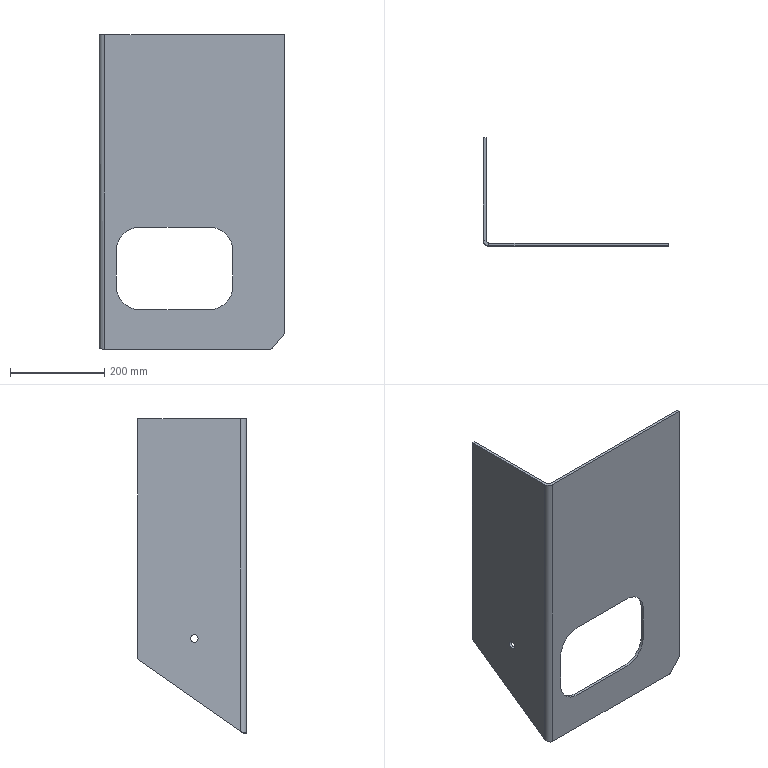Part | SolidWorks | features ICE 3, Chamfer 1, Fillet 1, FlatPattern 1, SMBaseFlange 1, SheetMetal 1 | 1 solid | 28 faces | box 394 x 230 x 667.799 mm | volume 2103650 mm3 | plane 16 | cylinder 11 | spline 1 | commonest cylinder face diameters 100 x4 15 x3 16 x2 12 x1 24 x1
STEP:
#1=CARTESIAN_POINT('',(6.,110.,-122.6));
#2=VERTEX_POINT('',#1);
#3=CARTESIAN_POINT('',(6.,110.,-138.6));
#4=VERTEX_POINT('',#3);
#5=CARTESIAN_POINT('',(6.,110.,-130.6));
#6=DIRECTION('',(1.,0.,0.));
#7=DIRECTION('',(0.,0.,-1.));
#8=AXIS2_PLACEMENT_3D('',#5,#6,#7);
#9=CIRCLE('',#8,8.);
#10=EDGE_CURVE('',#2,#4,#9,.T.);
#11=ORIENTED_EDGE('',*,*,#10,.T.);
#12=CARTESIAN_POINT('',(0.,110.,-138.6));
#13=VERTEX_POINT('',#12);
#14=CARTESIAN_POINT('',(10.,110.,-138.6));
#15=DIRECTION('',(-1.,0.,0.));
#16=VECTOR('',#15,1000.);
#17=LINE('',#14,#16);
#18=EDGE_CURVE('',#4,#13,#17,.T.);
#19=ORIENTED_EDGE('',*,*,#18,.T.);
#20=CARTESIAN_POINT('',(0.,110.,-122.6));
#21=VERTEX_POINT('',#20);
#22=CARTESIAN_POINT('',(0.,110.,-130.6));
#23=DIRECTION('',(-1.,0.,0.));
#24=DIRECTION('',(0.,0.,1.));
#25=AXIS2_PLACEMENT_3D('',#22,#23,#24);
#26=CIRCLE('',#25,8.);
#27=EDGE_CURVE('',#13,#21,#26,.T.);
#28=ORIENTED_EDGE('',*,*,#27,.T.);
#29=CARTESIAN_POINT('',(10.,110.,-122.6));
#30=DIRECTION('',(-1.,0.,0.));
#31=VECTOR('',#30,1000.);
#32=LINE('',#29,#31);
#33=EDGE_CURVE('',#2,#21,#32,.T.);
#34=ORIENTED_EDGE('',*,*,#33,.F.);
#35=EDGE_LOOP('',(#11,#19,#28,#34));
#36=FACE_OUTER_BOUND('',#35,.T.);
#37=CARTESIAN_POINT('',(10.,110.,-130.6));
#38=DIRECTION('',(-1.,0.,0.));
#39=DIRECTION('',(0.,0.,1.));
#40=AXIS2_PLACEMENT_3D('',#37,#38,#39);
#41=CYLINDRICAL_SURFACE('',#40,8.);
#42=ADVANCED_FACE('',(#36),#41,.F.);
#43=CARTESIAN_POINT('',(284.,0.,-197.7));
#44=VERTEX_POINT('',#43);
#45=CARTESIAN_POINT('',(284.,0.,-122.7));
#46=VERTEX_POINT('',#45);
#47=CARTESIAN_POINT('',(284.,0.,-197.7));
#48=DIRECTION('',(0.,0.,1.));
#49=VECTOR('',#48,1000.);
#50=LINE('',#47,#49);
#51=EDGE_CURVE('',#44,#46,#50,.T.);
#52=ORIENTED_EDGE('',*,*,#51,.F.);
#53=CARTESIAN_POINT('',(234.,0.,-247.7));
#54=VERTEX_POINT('',#53);
#55=CARTESIAN_POINT('',(234.,0.,-197.7));
#56=DIRECTION('',(0.,-1.,0.));
#57=DIRECTION('',(0.,0.,-1.));
#58=AXIS2_PLACEMENT_3D('',#55,#56,#57);
#59=CIRCLE('',#58,50.);
#60=EDGE_CURVE('',#54,#44,#59,.T.);
#61=ORIENTED_EDGE('',*,*,#60,.F.);
#62=CARTESIAN_POINT('',(86.,0.,-247.7));
#63=VERTEX_POINT('',#62);
#64=CARTESIAN_POINT('',(86.,0.,-247.7));
#65=DIRECTION('',(1.,0.,0.));
#66=VECTOR('',#65,1000.);
#67=LINE('',#64,#66);
#68=EDGE_CURVE('',#63,#54,#67,.T.);
#69=ORIENTED_EDGE('',*,*,#68,.F.);
#70=CARTESIAN_POINT('',(36.,0.,-197.7));
#71=VERTEX_POINT('',#70);
#72=CARTESIAN_POINT('',(86.,0.,-197.7));
#73=DIRECTION('',(0.,-1.,0.));
#74=DIRECTION('',(0.,0.,1.));
#75=AXIS2_PLACEMENT_3D('',#72,#73,#74);
#76=CIRCLE('',#75,50.);
#77=EDGE_CURVE('',#71,#63,#76,.T.);
#78=ORIENTED_EDGE('',*,*,#77,.F.);
#79=CARTESIAN_POINT('',(36.,0.,-122.7));
#80=VERTEX_POINT('',#79);
#81=CARTESIAN_POINT('',(36.,0.,-197.7));
#82=DIRECTION('',(0.,0.,-1.));
#83=VECTOR('',#82,1000.);
#84=LINE('',#81,#83);
#85=EDGE_CURVE('',#80,#71,#84,.T.);
#86=ORIENTED_EDGE('',*,*,#85,.F.);
#87=CARTESIAN_POINT('',(86.,0.,-72.7));
#88=VERTEX_POINT('',#87);
#89=CARTESIAN_POINT('',(86.,0.,-122.7));
#90=DIRECTION('',(0.,-1.,0.));
#91=DIRECTION('',(0.,0.,1.));
#92=AXIS2_PLACEMENT_3D('',#89,#90,#91);
#93=CIRCLE('',#92,50.);
#94=EDGE_CURVE('',#88,#80,#93,.T.);
#95=ORIENTED_EDGE('',*,*,#94,.F.);
#96=CARTESIAN_POINT('',(234.,0.,-72.7));
#97=VERTEX_POINT('',#96);
#98=CARTESIAN_POINT('',(86.,0.,-72.7));
#99=DIRECTION('',(-1.,0.,0.));
#100=VECTOR('',#99,1000.);
#101=LINE('',#98,#100);
#102=EDGE_CURVE('',#97,#88,#101,.T.);
#103=ORIENTED_EDGE('',*,*,#102,.F.);
#104=CARTESIAN_POINT('',(234.,0.,-122.7));
#105=DIRECTION('',(0.,-1.,0.));
#106=DIRECTION('',(0.,0.,1.));
#107=AXIS2_PLACEMENT_3D('',#104,#105,#106);
#108=CIRCLE('',#107,50.);
#109=EDGE_CURVE('',#46,#97,#108,.T.);
#110=ORIENTED_EDGE('',*,*,#109,.F.);
#111=EDGE_LOOP('',(#52,#61,#69,#78,#86,#95,#103,#110));
#112=FACE_BOUND('',#111,.T.);
#113=CARTESIAN_POINT('',(368.25,0.,-329.067));
#114=VERTEX_POINT('',#113);
#115=CARTESIAN_POINT('',(392.289,0.,-299.876));
#116=VERTEX_POINT('',#115);
#117=CARTESIAN_POINT('',(366.,0.,-331.799));
#118=DIRECTION('',(0.6357,0.,0.7719));
#119=VECTOR('',#118,1000.);
#120=LINE('',#117,#119);
#121=EDGE_CURVE('',#114,#116,#120,.T.);
#122=ORIENTED_EDGE('',*,*,#121,.T.);
#123=CARTESIAN_POINT('',(394.,0.,-295.108));
#124=VERTEX_POINT('',#123);
#125=CARTESIAN_POINT('',(386.5,0.,-295.108));
#126=DIRECTION('',(0.,-1.,0.));
#127=DIRECTION('',(0.,0.,1.));
#128=AXIS2_PLACEMENT_3D('',#125,#126,#127);
#129=CIRCLE('',#128,7.5);
#130=EDGE_CURVE('',#116,#124,#129,.T.);
#131=ORIENTED_EDGE('',*,*,#130,.T.);
#132=CARTESIAN_POINT('',(394.,0.,336.));
#133=VERTEX_POINT('',#132);
#134=CARTESIAN_POINT('',(394.,0.,336.));
#135=DIRECTION('',(0.,0.,-1.));
#136=VECTOR('',#135,1000.);
#137=LINE('',#134,#136);
#138=EDGE_CURVE('',#133,#124,#137,.T.);
#139=ORIENTED_EDGE('',*,*,#138,.F.);
#140=CARTESIAN_POINT('',(12.,0.,336.));
#141=VERTEX_POINT('',#140);
#142=CARTESIAN_POINT('',(0.,0.,336.));
#143=DIRECTION('',(1.,0.,0.));
#144=VECTOR('',#143,1000.);
#145=LINE('',#142,#144);
#146=EDGE_CURVE('',#141,#133,#145,.T.);
#147=ORIENTED_EDGE('',*,*,#146,.F.);
#148=CARTESIAN_POINT('',(12.,0.,-331.799));
#149=VERTEX_POINT('',#148);
#150=CARTESIAN_POINT('',(12.,0.,336.));
#151=DIRECTION('',(0.,0.,-1.));
#152=VECTOR('',#151,1000.);
#153=LINE('',#150,#152);
#154=EDGE_CURVE('',#141,#149,#153,.T.);
#155=ORIENTED_EDGE('',*,*,#154,.T.);
#156=CARTESIAN_POINT('',(362.461,0.,-331.799));
#157=VERTEX_POINT('',#156);
#158=CARTESIAN_POINT('',(0.,0.,-331.799));
#159=DIRECTION('',(1.,0.,0.));
#160=VECTOR('',#159,1000.);
#161=LINE('',#158,#160);
#162=EDGE_CURVE('',#149,#157,#161,.T.);
#163=ORIENTED_EDGE('',*,*,#162,.T.);
#164=CARTESIAN_POINT('',(362.461,0.,-324.299));
#165=DIRECTION('',(0.,-1.,0.));
#166=DIRECTION('',(0.,0.,1.));
#167=AXIS2_PLACEMENT_3D('',#164,#165,#166);
#168=CIRCLE('',#167,7.5);
#169=EDGE_CURVE('',#157,#114,#168,.T.);
#170=ORIENTED_EDGE('',*,*,#169,.T.);
#171=EDGE_LOOP('',(#122,#131,#139,#147,#155,#163,#170));
#172=FACE_OUTER_BOUND('',#171,.T.);
#173=CARTESIAN_POINT('',(0.,0.,336.));
#174=DIRECTION('',(0.,1.,0.));
#175=DIRECTION('',(0.,0.,1.));
#176=AXIS2_PLACEMENT_3D('',#173,#174,#175);
#177=PLANE('',#176);
#178=ADVANCED_FACE('',(#112,#172),#177,.F.);
#179=ORIENTED_EDGE('',*,*,#138,.T.);
#180=CARTESIAN_POINT('',(394.,6.,-295.108));
#181=VERTEX_POINT('',#180);
#182=CARTESIAN_POINT('',(394.,6.,-295.108));
#183=DIRECTION('',(0.,1.,0.));
#184=VECTOR('',#183,1000.);
#185=LINE('',#182,#184);
#186=EDGE_CURVE('',#124,#181,#185,.T.);
#187=ORIENTED_EDGE('',*,*,#186,.T.);
#188=CARTESIAN_POINT('',(394.,6.,336.));
#189=VERTEX_POINT('',#188);
#190=CARTESIAN_POINT('',(394.,6.,336.));
#191=DIRECTION('',(0.,0.,-1.));
#192=VECTOR('',#191,1000.);
#193=LINE('',#190,#192);
#194=EDGE_CURVE('',#189,#181,#193,.T.);
#195=ORIENTED_EDGE('',*,*,#194,.F.);
#196=CARTESIAN_POINT('',(394.,6.,336.));
#197=DIRECTION('',(0.,-1.,0.));
#198=VECTOR('',#197,1000.);
#199=LINE('',#196,#198);
#200=EDGE_CURVE('',#189,#133,#199,.T.);
#201=ORIENTED_EDGE('',*,*,#200,.T.);
#202=EDGE_LOOP('',(#179,#187,#195,#201));
#203=FACE_OUTER_BOUND('',#202,.T.);
#204=CARTESIAN_POINT('',(394.,6.,336.));
#205=DIRECTION('',(1.,0.,0.));
#206=DIRECTION('',(0.,0.,-1.));
#207=AXIS2_PLACEMENT_3D('',#204,#205,#206);
#208=PLANE('',#207);
#209=ADVANCED_FACE('',(#203),#208,.T.);
#210=CARTESIAN_POINT('',(284.,6.,-197.7));
#211=VERTEX_POINT('',#210);
#212=CARTESIAN_POINT('',(234.,6.,-247.7));
#213=VERTEX_POINT('',#212);
#214=CARTESIAN_POINT('',(234.,6.,-197.7));
#215=DIRECTION('',(0.,1.,0.));
#216=DIRECTION('',(0.,0.,1.));
#217=AXIS2_PLACEMENT_3D('',#214,#215,#216);
#218=CIRCLE('',#217,50.);
#219=EDGE_CURVE('',#211,#213,#218,.T.);
#220=ORIENTED_EDGE('',*,*,#219,.F.);
#221=CARTESIAN_POINT('',(284.,6.,-122.7));
#222=VERTEX_POINT('',#221);
#223=CARTESIAN_POINT('',(284.,6.,336.));
#224=DIRECTION('',(0.,0.,-1.));
#225=VECTOR('',#224,1000.);
#226=LINE('',#223,#225);
#227=EDGE_CURVE('',#222,#211,#226,.T.);
#228=ORIENTED_EDGE('',*,*,#227,.F.);
#229=CARTESIAN_POINT('',(234.,6.,-72.7));
#230=VERTEX_POINT('',#229);
#231=CARTESIAN_POINT('',(234.,6.,-122.7));
#232=DIRECTION('',(0.,1.,0.));
#233=DIRECTION('',(0.,0.,1.));
#234=AXIS2_PLACEMENT_3D('',#231,#232,#233);
#235=CIRCLE('',#234,50.);
#236=EDGE_CURVE('',#230,#222,#235,.T.);
#237=ORIENTED_EDGE('',*,*,#236,.F.);
#238=CARTESIAN_POINT('',(86.,6.,-72.7));
#239=VERTEX_POINT('',#238);
#240=CARTESIAN_POINT('',(0.,6.,-72.7));
#241=DIRECTION('',(1.,0.,0.));
#242=VECTOR('',#241,1000.);
#243=LINE('',#240,#242);
#244=EDGE_CURVE('',#239,#230,#243,.T.);
#245=ORIENTED_EDGE('',*,*,#244,.F.);
#246=CARTESIAN_POINT('',(36.,6.,-122.7));
#247=VERTEX_POINT('',#246);
#248=CARTESIAN_POINT('',(86.,6.,-122.7));
#249=DIRECTION('',(0.,1.,0.));
#250=DIRECTION('',(0.,0.,1.));
#251=AXIS2_PLACEMENT_3D('',#248,#249,#250);
#252=CIRCLE('',#251,50.);
#253=EDGE_CURVE('',#247,#239,#252,.T.);
#254=ORIENTED_EDGE('',*,*,#253,.F.);
#255=CARTESIAN_POINT('',(36.,6.,-197.7));
#256=VERTEX_POINT('',#255);
#257=CARTESIAN_POINT('',(36.,6.,336.));
#258=DIRECTION('',(0.,0.,1.));
#259=VECTOR('',#258,1000.);
#260=LINE('',#257,#259);
#261=EDGE_CURVE('',#256,#247,#260,.T.);
#262=ORIENTED_EDGE('',*,*,#261,.F.);
#263=CARTESIAN_POINT('',(86.,6.,-247.7));
#264=VERTEX_POINT('',#263);
#265=CARTESIAN_POINT('',(86.,6.,-197.7));
#266=DIRECTION('',(0.,1.,0.));
#267=DIRECTION('',(0.,0.,1.));
#268=AXIS2_PLACEMENT_3D('',#265,#266,#267);
#269=CIRCLE('',#268,50.);
#270=EDGE_CURVE('',#264,#256,#269,.T.);
#271=ORIENTED_EDGE('',*,*,#270,.F.);
#272=CARTESIAN_POINT('',(0.,6.,-247.7));
#273=DIRECTION('',(-1.,0.,0.));
#274=VECTOR('',#273,1000.);
#275=LINE('',#272,#274);
#276=EDGE_CURVE('',#213,#264,#275,.T.);
#277=ORIENTED_EDGE('',*,*,#276,.F.);
#278=EDGE_LOOP('',(#220,#228,#237,#245,#254,#262,#271,#277));
#279=FACE_BOUND('',#278,.T.);
#280=ORIENTED_EDGE('',*,*,#194,.T.);
#281=CARTESIAN_POINT('',(392.289,6.,-299.876));
#282=VERTEX_POINT('',#281);
#283=CARTESIAN_POINT('',(386.5,6.,-295.108));
#284=DIRECTION('',(0.,1.,0.));
#285=DIRECTION('',(0.,0.,1.));
#286=AXIS2_PLACEMENT_3D('',#283,#284,#285);
#287=CIRCLE('',#286,7.5);
#288=EDGE_CURVE('',#181,#282,#287,.T.);
#289=ORIENTED_EDGE('',*,*,#288,.T.);
#290=CARTESIAN_POINT('',(368.25,6.,-329.067));
#291=VERTEX_POINT('',#290);
#292=CARTESIAN_POINT('',(545.794,6.,-113.477));
#293=DIRECTION('',(-0.6357,0.,-0.7719));
#294=VECTOR('',#293,1000.);
#295=LINE('',#292,#294);
#296=EDGE_CURVE('',#282,#291,#295,.T.);
#297=ORIENTED_EDGE('',*,*,#296,.T.);
#298=CARTESIAN_POINT('',(362.461,6.,-331.799));
#299=VERTEX_POINT('',#298);
#300=CARTESIAN_POINT('',(362.461,6.,-324.299));
#301=DIRECTION('',(0.,1.,0.));
#302=DIRECTION('',(0.,0.,1.));
#303=AXIS2_PLACEMENT_3D('',#300,#301,#302);
#304=CIRCLE('',#303,7.5);
#305=EDGE_CURVE('',#291,#299,#304,.T.);
#306=ORIENTED_EDGE('',*,*,#305,.T.);
#307=CARTESIAN_POINT('',(12.,6.,-331.799));
#308=VERTEX_POINT('',#307);
#309=CARTESIAN_POINT('',(0.,6.,-331.799));
#310=DIRECTION('',(1.,0.,0.));
#311=VECTOR('',#310,1000.);
#312=LINE('',#309,#311);
#313=EDGE_CURVE('',#308,#299,#312,.T.);
#314=ORIENTED_EDGE('',*,*,#313,.F.);
#315=CARTESIAN_POINT('',(12.,6.,336.));
#316=VERTEX_POINT('',#315);
#317=CARTESIAN_POINT('',(12.,6.,336.));
#318=DIRECTION('',(0.,0.,-1.));
#319=VECTOR('',#318,1000.);
#320=LINE('',#317,#319);
#321=EDGE_CURVE('',#316,#308,#320,.T.);
#322=ORIENTED_EDGE('',*,*,#321,.F.);
#323=CARTESIAN_POINT('',(0.,6.,336.));
#324=DIRECTION('',(1.,0.,0.));
#325=VECTOR('',#324,1000.);
#326=LINE('',#323,#325);
#327=EDGE_CURVE('',#316,#189,#326,.T.);
#328=ORIENTED_EDGE('',*,*,#327,.T.);
#329=EDGE_LOOP('',(#280,#289,#297,#306,#314,#322,#328));
#330=FACE_OUTER_BOUND('',#329,.T.);
#331=CARTESIAN_POINT('',(0.,6.,336.));
#332=DIRECTION('',(0.,1.,0.));
#333=DIRECTION('',(0.,0.,1.));
#334=AXIS2_PLACEMENT_3D('',#331,#332,#333);
#335=PLANE('',#334);
#336=ADVANCED_FACE('',(#279,#330),#335,.T.);
#337=ORIENTED_EDGE('',*,*,#321,.T.);
#338=CARTESIAN_POINT('',(6.,12.,-327.598));
#339=VERTEX_POINT('',#338);
#340=CARTESIAN_POINT('',(6.,12.,-327.598));
#341=CARTESIAN_POINT('',(6.,8.485,-330.059));
#342=CARTESIAN_POINT('',(8.485,6.,-331.799));
#343=CARTESIAN_POINT('',(12.,6.,-331.799));
#344=(BOUNDED_CURVE()B_SPLINE_CURVE(3,(#340,#341,#342,#343),.UNSPECIFIED.,.F.,.T.)B_SPLINE_CURVE_WITH_KNOTS((4,4),(4.712,6.283),.UNSPECIFIED.)CURVE()GEOMETRIC_REPRESENTATION_ITEM()RATIONAL_B_SPLINE_CURVE((1.,0.8047,0.8047,1.))REPRESENTATION_ITEM(''));
#345=EDGE_CURVE('',#339,#308,#344,.T.);
#346=ORIENTED_EDGE('',*,*,#345,.F.);
#347=CARTESIAN_POINT('',(6.,12.,336.));
#348=VERTEX_POINT('',#347);
#349=CARTESIAN_POINT('',(6.,12.,336.));
#350=DIRECTION('',(0.,0.,-1.));
#351=VECTOR('',#350,1000.);
#352=LINE('',#349,#351);
#353=EDGE_CURVE('',#348,#339,#352,.T.);
#354=ORIENTED_EDGE('',*,*,#353,.F.);
#355=CARTESIAN_POINT('',(12.,12.,336.));
#356=DIRECTION('',(0.,0.,1.));
#357=DIRECTION('',(1.,0.,0.));
#358=AXIS2_PLACEMENT_3D('',#355,#356,#357);
#359=CIRCLE('',#358,6.);
#360=EDGE_CURVE('',#348,#316,#359,.T.);
#361=ORIENTED_EDGE('',*,*,#360,.T.);
#362=EDGE_LOOP('',(#337,#346,#354,#361));
#363=FACE_OUTER_BOUND('',#362,.T.);
#364=CARTESIAN_POINT('',(12.,12.,336.));
#365=DIRECTION('',(0.,0.,-1.));
#366=DIRECTION('',(-1.,0.,0.));
#367=AXIS2_PLACEMENT_3D('',#364,#365,#366);
#368=CYLINDRICAL_SURFACE('',#367,6.);
#369=ADVANCED_FACE('',(#363),#368,.F.);
#370=ORIENTED_EDGE('',*,*,#10,.F.);
#371=CARTESIAN_POINT('',(6.,110.,-130.6));
#372=DIRECTION('',(1.,0.,0.));
#373=DIRECTION('',(0.,0.,-1.));
#374=AXIS2_PLACEMENT_3D('',#371,#372,#373);
#375=CIRCLE('',#374,8.);
#376=EDGE_CURVE('',#4,#2,#375,.T.);
#377=ORIENTED_EDGE('',*,*,#376,.F.);
#378=EDGE_LOOP('',(#370,#377));
#379=FACE_BOUND('',#378,.T.);
#380=CARTESIAN_POINT('',(6.,226.802,-177.192));
#381=VERTEX_POINT('',#380);
#382=CARTESIAN_POINT('',(6.,315.737,-114.919));
#383=DIRECTION('',(0.,-0.8192,-0.5736));
#384=VECTOR('',#383,1000.);
#385=LINE('',#382,#384);
#386=EDGE_CURVE('',#381,#339,#385,.T.);
#387=ORIENTED_EDGE('',*,*,#386,.F.);
#388=CARTESIAN_POINT('',(6.,230.,-171.048));
#389=VERTEX_POINT('',#388);
#390=CARTESIAN_POINT('',(6.,222.5,-171.048));
#391=DIRECTION('',(1.,0.,0.));
#392=DIRECTION('',(0.,0.,-1.));
#393=AXIS2_PLACEMENT_3D('',#390,#391,#392);
#394=CIRCLE('',#393,7.5);
#395=EDGE_CURVE('',#381,#389,#394,.T.);
#396=ORIENTED_EDGE('',*,*,#395,.T.);
#397=CARTESIAN_POINT('',(6.,230.,336.));
#398=VERTEX_POINT('',#397);
#399=CARTESIAN_POINT('',(6.,230.,336.));
#400=DIRECTION('',(0.,0.,-1.));
#401=VECTOR('',#400,1000.);
#402=LINE('',#399,#401);
#403=EDGE_CURVE('',#398,#389,#402,.T.);
#404=ORIENTED_EDGE('',*,*,#403,.F.);
#405=CARTESIAN_POINT('',(6.,0.,336.));
#406=DIRECTION('',(0.,-1.,0.));
#407=VECTOR('',#406,1000.);
#408=LINE('',#405,#407);
#409=EDGE_CURVE('',#398,#348,#408,.T.);
#410=ORIENTED_EDGE('',*,*,#409,.T.);
#411=ORIENTED_EDGE('',*,*,#353,.T.);
#412=EDGE_LOOP('',(#387,#396,#404,#410,#411));
#413=FACE_OUTER_BOUND('',#412,.T.);
#414=CARTESIAN_POINT('',(6.,0.,336.));
#415=DIRECTION('',(1.,0.,0.));
#416=DIRECTION('',(0.,0.,-1.));
#417=AXIS2_PLACEMENT_3D('',#414,#415,#416);
#418=PLANE('',#417);
#419=ADVANCED_FACE('',(#379,#413),#418,.T.);
#420=ORIENTED_EDGE('',*,*,#403,.T.);
#421=CARTESIAN_POINT('',(0.,230.,-171.048));
#422=VERTEX_POINT('',#421);
#423=CARTESIAN_POINT('',(0.,230.,-171.048));
#424=DIRECTION('',(-1.,0.,0.));
#425=VECTOR('',#424,1000.);
#426=LINE('',#423,#425);
#427=EDGE_CURVE('',#389,#422,#426,.T.);
#428=ORIENTED_EDGE('',*,*,#427,.T.);
#429=CARTESIAN_POINT('',(0.,230.,336.));
#430=VERTEX_POINT('',#429);
#431=CARTESIAN_POINT('',(0.,230.,336.));
#432=DIRECTION('',(0.,0.,-1.));
#433=VECTOR('',#432,1000.);
#434=LINE('',#431,#433);
#435=EDGE_CURVE('',#430,#422,#434,.T.);
#436=ORIENTED_EDGE('',*,*,#435,.F.);
#437=CARTESIAN_POINT('',(0.,230.,336.));
#438=DIRECTION('',(1.,0.,0.));
#439=VECTOR('',#438,1000.);
#440=LINE('',#437,#439);
#441=EDGE_CURVE('',#430,#398,#440,.T.);
#442=ORIENTED_EDGE('',*,*,#441,.T.);
#443=EDGE_LOOP('',(#420,#428,#436,#442));
#444=FACE_OUTER_BOUND('',#443,.T.);
#445=CARTESIAN_POINT('',(0.,230.,336.));
#446=DIRECTION('',(0.,1.,0.));
#447=DIRECTION('',(0.,0.,1.));
#448=AXIS2_PLACEMENT_3D('',#445,#446,#447);
#449=PLANE('',#448);
#450=ADVANCED_FACE('',(#444),#449,.T.);
#451=CARTESIAN_POINT('',(0.,110.,-130.6));
#452=DIRECTION('',(-1.,0.,0.));
#453=DIRECTION('',(0.,0.,1.));
#454=AXIS2_PLACEMENT_3D('',#451,#452,#453);
#455=CIRCLE('',#454,8.);
#456=EDGE_CURVE('',#21,#13,#455,.T.);
#457=ORIENTED_EDGE('',*,*,#456,.F.);
#458=ORIENTED_EDGE('',*,*,#27,.F.);
#459=EDGE_LOOP('',(#457,#458));
#460=FACE_BOUND('',#459,.T.);
#461=ORIENTED_EDGE('',*,*,#435,.T.);
#462=CARTESIAN_POINT('',(0.,226.802,-177.192));
#463=VERTEX_POINT('',#462);
#464=CARTESIAN_POINT('',(0.,222.5,-171.048));
#465=DIRECTION('',(-1.,0.,0.));
#466=DIRECTION('',(0.,0.,-1.));
#467=AXIS2_PLACEMENT_3D('',#464,#465,#466);
#468=CIRCLE('',#467,7.5);
#469=EDGE_CURVE('',#422,#463,#468,.T.);
#470=ORIENTED_EDGE('',*,*,#469,.T.);
#471=CARTESIAN_POINT('',(0.,12.,-327.598));
#472=VERTEX_POINT('',#471);
#473=CARTESIAN_POINT('',(0.,315.737,-114.919));
#474=DIRECTION('',(0.,-0.8192,-0.5736));
#475=VECTOR('',#474,1000.);
#476=LINE('',#473,#475);
#477=EDGE_CURVE('',#463,#472,#476,.T.);
#478=ORIENTED_EDGE('',*,*,#477,.T.);
#479=CARTESIAN_POINT('',(0.,12.,336.));
#480=VERTEX_POINT('',#479);
#481=CARTESIAN_POINT('',(0.,12.,336.));
#482=DIRECTION('',(0.,0.,-1.));
#483=VECTOR('',#482,1000.);
#484=LINE('',#481,#483);
#485=EDGE_CURVE('',#480,#472,#484,.T.);
#486=ORIENTED_EDGE('',*,*,#485,.F.);
#487=CARTESIAN_POINT('',(0.,0.,336.));
#488=DIRECTION('',(0.,-1.,0.));
#489=VECTOR('',#488,1000.);
#490=LINE('',#487,#489);
#491=EDGE_CURVE('',#430,#480,#490,.T.);
#492=ORIENTED_EDGE('',*,*,#491,.F.);
#493=EDGE_LOOP('',(#461,#470,#478,#486,#492));
#494=FACE_OUTER_BOUND('',#493,.T.);
#495=CARTESIAN_POINT('',(0.,0.,336.));
#496=DIRECTION('',(1.,0.,0.));
#497=DIRECTION('',(0.,0.,-1.));
#498=AXIS2_PLACEMENT_3D('',#495,#496,#497);
#499=PLANE('',#498);
#500=ADVANCED_FACE('',(#460,#494),#499,.F.);
#501=CARTESIAN_POINT('',(0.,12.,-327.598));
#502=CARTESIAN_POINT('',(0.,4.971,-330.059));
#503=CARTESIAN_POINT('',(4.971,0.,-331.799));
#504=CARTESIAN_POINT('',(12.,0.,-331.799));
#505=(BOUNDED_CURVE()B_SPLINE_CURVE(3,(#501,#502,#503,#504),.UNSPECIFIED.,.F.,.F.)B_SPLINE_CURVE_WITH_KNOTS((4,4),(4.712,6.283),.UNSPECIFIED.)CURVE()GEOMETRIC_REPRESENTATION_ITEM()RATIONAL_B_SPLINE_CURVE((1.,0.8047,0.8047,1.))REPRESENTATION_ITEM(''));
#506=EDGE_CURVE('',#472,#149,#505,.T.);
#507=ORIENTED_EDGE('',*,*,#506,.T.);
#508=ORIENTED_EDGE('',*,*,#154,.F.);
#509=CARTESIAN_POINT('',(12.,12.,336.));
#510=DIRECTION('',(0.,0.,1.));
#511=DIRECTION('',(-1.,0.,0.));
#512=AXIS2_PLACEMENT_3D('',#509,#510,#511);
#513=CIRCLE('',#512,12.);
#514=EDGE_CURVE('',#480,#141,#513,.T.);
#515=ORIENTED_EDGE('',*,*,#514,.F.);
#516=ORIENTED_EDGE('',*,*,#485,.T.);
#517=EDGE_LOOP('',(#507,#508,#515,#516));
#518=FACE_OUTER_BOUND('',#517,.T.);
#519=CARTESIAN_POINT('',(12.,12.,336.));
#520=DIRECTION('',(0.,0.,-1.));
#521=DIRECTION('',(-1.,0.,0.));
#522=AXIS2_PLACEMENT_3D('',#519,#520,#521);
#523=CYLINDRICAL_SURFACE('',#522,12.);
#524=ADVANCED_FACE('',(#518),#523,.T.);
#525=CARTESIAN_POINT('',(0.,12.,336.));
#526=DIRECTION('',(1.,0.,0.));
#527=VECTOR('',#526,1000.);
#528=LINE('',#525,#527);
#529=EDGE_CURVE('',#480,#348,#528,.T.);
#530=ORIENTED_EDGE('',*,*,#529,.F.);
#531=ORIENTED_EDGE('',*,*,#514,.T.);
#532=CARTESIAN_POINT('',(12.,6.,336.));
#533=DIRECTION('',(0.,-1.,0.));
#534=VECTOR('',#533,1000.);
#535=LINE('',#532,#534);
#536=EDGE_CURVE('',#316,#141,#535,.T.);
#537=ORIENTED_EDGE('',*,*,#536,.F.);
#538=ORIENTED_EDGE('',*,*,#360,.F.);
#539=EDGE_LOOP('',(#530,#531,#537,#538));
#540=FACE_OUTER_BOUND('',#539,.T.);
#541=CARTESIAN_POINT('',(0.,12.,336.));
#542=DIRECTION('',(0.,0.,1.));
#543=DIRECTION('',(1.,0.,0.));
#544=AXIS2_PLACEMENT_3D('',#541,#542,#543);
#545=PLANE('',#544);
#546=ADVANCED_FACE('',(#540),#545,.T.);
#547=ORIENTED_EDGE('',*,*,#491,.T.);
#548=ORIENTED_EDGE('',*,*,#529,.T.);
#549=ORIENTED_EDGE('',*,*,#409,.F.);
#550=ORIENTED_EDGE('',*,*,#441,.F.);
#551=EDGE_LOOP('',(#547,#548,#549,#550));
#552=FACE_OUTER_BOUND('',#551,.T.);
#553=CARTESIAN_POINT('',(12.,6.,336.));
#554=DIRECTION('',(0.,0.,1.));
#555=DIRECTION('',(1.,0.,0.));
#556=AXIS2_PLACEMENT_3D('',#553,#554,#555);
#557=PLANE('',#556);
#558=ADVANCED_FACE('',(#552),#557,.T.);
#559=ORIENTED_EDGE('',*,*,#146,.T.);
#560=ORIENTED_EDGE('',*,*,#200,.F.);
#561=ORIENTED_EDGE('',*,*,#327,.F.);
#562=ORIENTED_EDGE('',*,*,#536,.T.);
#563=EDGE_LOOP('',(#559,#560,#561,#562));
#564=FACE_OUTER_BOUND('',#563,.T.);
#565=CARTESIAN_POINT('',(12.,12.,336.));
#566=DIRECTION('',(0.,0.,1.));
#567=DIRECTION('',(1.,0.,0.));
#568=AXIS2_PLACEMENT_3D('',#565,#566,#567);
#569=PLANE('',#568);
#570=ADVANCED_FACE('',(#564),#569,.T.);
#571=ORIENTED_EDGE('',*,*,#313,.T.);
#572=CARTESIAN_POINT('',(362.461,6.,-331.799));
#573=DIRECTION('',(0.,-1.,0.));
#574=VECTOR('',#573,1000.);
#575=LINE('',#572,#574);
#576=EDGE_CURVE('',#299,#157,#575,.T.);
#577=ORIENTED_EDGE('',*,*,#576,.T.);
#578=ORIENTED_EDGE('',*,*,#162,.F.);
#579=CARTESIAN_POINT('',(12.,6.,-331.799));
#580=DIRECTION('',(0.,-1.,0.));
#581=VECTOR('',#580,1000.);
#582=LINE('',#579,#581);
#583=EDGE_CURVE('',#308,#149,#582,.T.);
#584=ORIENTED_EDGE('',*,*,#583,.F.);
#585=EDGE_LOOP('',(#571,#577,#578,#584));
#586=FACE_OUTER_BOUND('',#585,.T.);
#587=CARTESIAN_POINT('',(0.,6.,-331.799));
#588=DIRECTION('',(0.,0.,1.));
#589=DIRECTION('',(1.,0.,0.));
#590=AXIS2_PLACEMENT_3D('',#587,#588,#589);
#591=PLANE('',#590);
#592=ADVANCED_FACE('',(#586),#591,.F.);
#593=ORIENTED_EDGE('',*,*,#477,.F.);
#594=CARTESIAN_POINT('',(6.,226.802,-177.192));
#595=DIRECTION('',(1.,0.,0.));
#596=VECTOR('',#595,1000.);
#597=LINE('',#594,#596);
#598=EDGE_CURVE('',#463,#381,#597,.T.);
#599=ORIENTED_EDGE('',*,*,#598,.T.);
#600=ORIENTED_EDGE('',*,*,#386,.T.);
#601=CARTESIAN_POINT('',(6.,12.,-327.598));
#602=DIRECTION('',(-1.,0.,0.));
#603=VECTOR('',#602,1000.);
#604=LINE('',#601,#603);
#605=EDGE_CURVE('',#339,#472,#604,.T.);
#606=ORIENTED_EDGE('',*,*,#605,.T.);
#607=EDGE_LOOP('',(#593,#599,#600,#606));
#608=FACE_OUTER_BOUND('',#607,.T.);
#609=CARTESIAN_POINT('',(6.,315.737,-114.919));
#610=DIRECTION('',(0.,-0.5736,0.8192));
#611=DIRECTION('',(0.,-0.8192,-0.5736));
#612=AXIS2_PLACEMENT_3D('',#609,#610,#611);
#613=PLANE('',#612);
#614=ADVANCED_FACE('',(#608),#613,.F.);
#615=ORIENTED_EDGE('',*,*,#345,.T.);
#616=ORIENTED_EDGE('',*,*,#583,.T.);
#617=ORIENTED_EDGE('',*,*,#506,.F.);
#618=ORIENTED_EDGE('',*,*,#605,.F.);
#619=EDGE_LOOP('',(#615,#616,#617,#618));
#620=FACE_OUTER_BOUND('',#619,.T.);
#621=CARTESIAN_POINT('',(12.,6.,-331.799));
#622=CARTESIAN_POINT('',(12.,4.,-331.799));
#623=CARTESIAN_POINT('',(12.,2.,-331.799));
#624=CARTESIAN_POINT('',(12.,0.,-331.799));
#625=CARTESIAN_POINT('',(24.,6.,-331.799));
#626=CARTESIAN_POINT('',(28.,4.,-331.799));
#627=CARTESIAN_POINT('',(32.,2.,-331.799));
#628=CARTESIAN_POINT('',(36.,0.,-331.799));
#629=CARTESIAN_POINT('',(24.,18.,-323.396));
#630=CARTESIAN_POINT('',(28.,20.,-323.396));
#631=CARTESIAN_POINT('',(32.,22.,-323.396));
#632=CARTESIAN_POINT('',(36.,24.,-323.396));
#633=CARTESIAN_POINT('',(12.,18.,-323.396));
#634=CARTESIAN_POINT('',(12.,20.,-323.396));
#635=CARTESIAN_POINT('',(12.,22.,-323.396));
#636=CARTESIAN_POINT('',(12.,24.,-323.396));
#637=CARTESIAN_POINT('',(0.,18.,-323.396));
#638=CARTESIAN_POINT('',(-4.,20.,-323.396));
#639=CARTESIAN_POINT('',(-8.,22.,-323.396));
#640=CARTESIAN_POINT('',(-12.,24.,-323.396));
#641=CARTESIAN_POINT('',(0.,6.,-331.799));
#642=CARTESIAN_POINT('',(-4.,4.,-331.799));
#643=CARTESIAN_POINT('',(-8.,2.,-331.799));
#644=CARTESIAN_POINT('',(-12.,0.,-331.799));
#645=CARTESIAN_POINT('',(12.,6.,-331.799));
#646=CARTESIAN_POINT('',(12.,4.,-331.799));
#647=CARTESIAN_POINT('',(12.,2.,-331.799));
#648=CARTESIAN_POINT('',(12.,0.,-331.799));
#649=(BOUNDED_SURFACE()B_SPLINE_SURFACE(3,3,((#621,#622,#623,#624),(#625,#626,#627,#628),(#629,#630,#631,#632),(#633,#634,#635,#636),(#637,#638,#639,#640),(#641,#642,#643,#644),(#645,#646,#647,#648)),.UNSPECIFIED.,.T.,.F.,.T.)B_SPLINE_SURFACE_WITH_KNOTS((4,3,4),(4,4),(0.,0.5,1.),(0.,1.),.UNSPECIFIED.)GEOMETRIC_REPRESENTATION_ITEM()RATIONAL_B_SPLINE_SURFACE(((1.,1.,1.,1.),(0.3333,0.3333,0.3333,0.3333),(0.3333,0.3333,0.3333,0.3333),(1.,1.,1.,1.),(0.3333,0.3333,0.3333,0.3333),(0.3333,0.3333,0.3333,0.3333),(1.,1.,1.,1.)))REPRESENTATION_ITEM('')SURFACE());
#650=ADVANCED_FACE('',(#620),#649,.T.);
#651=ORIENTED_EDGE('',*,*,#296,.F.);
#652=CARTESIAN_POINT('',(392.289,6.,-299.876));
#653=DIRECTION('',(0.,-1.,0.));
#654=VECTOR('',#653,1000.);
#655=LINE('',#652,#654);
#656=EDGE_CURVE('',#282,#116,#655,.T.);
#657=ORIENTED_EDGE('',*,*,#656,.T.);
#658=ORIENTED_EDGE('',*,*,#121,.F.);
#659=CARTESIAN_POINT('',(368.25,6.,-329.067));
#660=DIRECTION('',(0.,1.,0.));
#661=VECTOR('',#660,1000.);
#662=LINE('',#659,#661);
#663=EDGE_CURVE('',#114,#291,#662,.T.);
#664=ORIENTED_EDGE('',*,*,#663,.T.);
#665=EDGE_LOOP('',(#651,#657,#658,#664));
#666=FACE_OUTER_BOUND('',#665,.T.);
#667=CARTESIAN_POINT('',(366.,6.,-331.799));
#668=DIRECTION('',(0.7719,0.,-0.6357));
#669=DIRECTION('',(0.,1.,0.));
#670=AXIS2_PLACEMENT_3D('',#667,#668,#669);
#671=PLANE('',#670);
#672=ADVANCED_FACE('',(#666),#671,.T.);
#673=ORIENTED_EDGE('',*,*,#395,.F.);
#674=ORIENTED_EDGE('',*,*,#598,.F.);
#675=ORIENTED_EDGE('',*,*,#469,.F.);
#676=ORIENTED_EDGE('',*,*,#427,.F.);
#677=EDGE_LOOP('',(#673,#674,#675,#676));
#678=FACE_OUTER_BOUND('',#677,.T.);
#679=CARTESIAN_POINT('',(0.,222.5,-171.048));
#680=DIRECTION('',(1.,0.,0.));
#681=DIRECTION('',(0.,0.,-1.));
#682=AXIS2_PLACEMENT_3D('',#679,#680,#681);
#683=CYLINDRICAL_SURFACE('',#682,7.5);
#684=ADVANCED_FACE('',(#678),#683,.T.);
#685=ORIENTED_EDGE('',*,*,#130,.F.);
#686=ORIENTED_EDGE('',*,*,#656,.F.);
#687=ORIENTED_EDGE('',*,*,#288,.F.);
#688=ORIENTED_EDGE('',*,*,#186,.F.);
#689=EDGE_LOOP('',(#685,#686,#687,#688));
#690=FACE_OUTER_BOUND('',#689,.T.);
#691=CARTESIAN_POINT('',(386.5,6.,-295.108));
#692=DIRECTION('',(0.,1.,0.));
#693=DIRECTION('',(0.,0.,1.));
#694=AXIS2_PLACEMENT_3D('',#691,#692,#693);
#695=CYLINDRICAL_SURFACE('',#694,7.5);
#696=ADVANCED_FACE('',(#690),#695,.T.);
#697=ORIENTED_EDGE('',*,*,#305,.F.);
#698=ORIENTED_EDGE('',*,*,#663,.F.);
#699=ORIENTED_EDGE('',*,*,#169,.F.);
#700=ORIENTED_EDGE('',*,*,#576,.F.);
#701=EDGE_LOOP('',(#697,#698,#699,#700));
#702=FACE_OUTER_BOUND('',#701,.T.);
#703=CARTESIAN_POINT('',(362.461,6.,-324.299));
#704=DIRECTION('',(0.,1.,0.));
#705=DIRECTION('',(0.,0.,1.));
#706=AXIS2_PLACEMENT_3D('',#703,#704,#705);
#707=CYLINDRICAL_SURFACE('',#706,7.5);
#708=ADVANCED_FACE('',(#702),#707,.T.);
#709=ORIENTED_EDGE('',*,*,#18,.F.);
#710=ORIENTED_EDGE('',*,*,#376,.T.);
#711=ORIENTED_EDGE('',*,*,#33,.T.);
#712=ORIENTED_EDGE('',*,*,#456,.T.);
#713=EDGE_LOOP('',(#709,#710,#711,#712));
#714=FACE_OUTER_BOUND('',#713,.T.);
#715=CARTESIAN_POINT('',(10.,110.,-130.6));
#716=DIRECTION('',(-1.,0.,0.));
#717=DIRECTION('',(0.,0.,1.));
#718=AXIS2_PLACEMENT_3D('',#715,#716,#717);
#719=CYLINDRICAL_SURFACE('',#718,8.);
#720=ADVANCED_FACE('',(#714),#719,.F.);
#721=ORIENTED_EDGE('',*,*,#219,.T.);
#722=CARTESIAN_POINT('',(234.,10.,-247.7));
#723=DIRECTION('',(0.,-1.,0.));
#724=VECTOR('',#723,1000.);
#725=LINE('',#722,#724);
#726=EDGE_CURVE('',#213,#54,#725,.T.);
#727=ORIENTED_EDGE('',*,*,#726,.T.);
#728=ORIENTED_EDGE('',*,*,#60,.T.);
#729=CARTESIAN_POINT('',(284.,10.,-197.7));
#730=DIRECTION('',(0.,-1.,0.));
#731=VECTOR('',#730,1000.);
#732=LINE('',#729,#731);
#733=EDGE_CURVE('',#211,#44,#732,.T.);
#734=ORIENTED_EDGE('',*,*,#733,.F.);
#735=EDGE_LOOP('',(#721,#727,#728,#734));
#736=FACE_OUTER_BOUND('',#735,.T.);
#737=CARTESIAN_POINT('',(234.,10.,-197.7));
#738=DIRECTION('',(0.,-1.,0.));
#739=DIRECTION('',(0.,0.,-1.));
#740=AXIS2_PLACEMENT_3D('',#737,#738,#739);
#741=CYLINDRICAL_SURFACE('',#740,50.);
#742=ADVANCED_FACE('',(#736),#741,.F.);
#743=ORIENTED_EDGE('',*,*,#276,.T.);
#744=CARTESIAN_POINT('',(86.,10.,-247.7));
#745=DIRECTION('',(0.,-1.,0.));
#746=VECTOR('',#745,1000.);
#747=LINE('',#744,#746);
#748=EDGE_CURVE('',#264,#63,#747,.T.);
#749=ORIENTED_EDGE('',*,*,#748,.T.);
#750=ORIENTED_EDGE('',*,*,#68,.T.);
#751=ORIENTED_EDGE('',*,*,#726,.F.);
#752=EDGE_LOOP('',(#743,#749,#750,#751));
#753=FACE_OUTER_BOUND('',#752,.T.);
#754=CARTESIAN_POINT('',(86.,10.,-247.7));
#755=DIRECTION('',(0.,0.,-1.));
#756=DIRECTION('',(-1.,0.,0.));
#757=AXIS2_PLACEMENT_3D('',#754,#755,#756);
#758=PLANE('',#757);
#759=ADVANCED_FACE('',(#753),#758,.F.);
#760=ORIENTED_EDGE('',*,*,#270,.T.);
#761=CARTESIAN_POINT('',(36.,10.,-197.7));
#762=DIRECTION('',(0.,-1.,0.));
#763=VECTOR('',#762,1000.);
#764=LINE('',#761,#763);
#765=EDGE_CURVE('',#256,#71,#764,.T.);
#766=ORIENTED_EDGE('',*,*,#765,.T.);
#767=ORIENTED_EDGE('',*,*,#77,.T.);
#768=ORIENTED_EDGE('',*,*,#748,.F.);
#769=EDGE_LOOP('',(#760,#766,#767,#768));
#770=FACE_OUTER_BOUND('',#769,.T.);
#771=CARTESIAN_POINT('',(86.,10.,-197.7));
#772=DIRECTION('',(0.,-1.,0.));
#773=DIRECTION('',(0.,0.,-1.));
#774=AXIS2_PLACEMENT_3D('',#771,#772,#773);
#775=CYLINDRICAL_SURFACE('',#774,50.);
#776=ADVANCED_FACE('',(#770),#775,.F.);
#777=ORIENTED_EDGE('',*,*,#261,.T.);
#778=CARTESIAN_POINT('',(36.,10.,-122.7));
#779=DIRECTION('',(0.,-1.,0.));
#780=VECTOR('',#779,1000.);
#781=LINE('',#778,#780);
#782=EDGE_CURVE('',#247,#80,#781,.T.);
#783=ORIENTED_EDGE('',*,*,#782,.T.);
#784=ORIENTED_EDGE('',*,*,#85,.T.);
#785=ORIENTED_EDGE('',*,*,#765,.F.);
#786=EDGE_LOOP('',(#777,#783,#784,#785));
#787=FACE_OUTER_BOUND('',#786,.T.);
#788=CARTESIAN_POINT('',(36.,10.,-197.7));
#789=DIRECTION('',(-1.,0.,0.));
#790=DIRECTION('',(0.,0.,1.));
#791=AXIS2_PLACEMENT_3D('',#788,#789,#790);
#792=PLANE('',#791);
#793=ADVANCED_FACE('',(#787),#792,.F.);
#794=ORIENTED_EDGE('',*,*,#253,.T.);
#795=CARTESIAN_POINT('',(86.,10.,-72.7));
#796=DIRECTION('',(0.,-1.,0.));
#797=VECTOR('',#796,1000.);
#798=LINE('',#795,#797);
#799=EDGE_CURVE('',#239,#88,#798,.T.);
#800=ORIENTED_EDGE('',*,*,#799,.T.);
#801=ORIENTED_EDGE('',*,*,#94,.T.);
#802=ORIENTED_EDGE('',*,*,#782,.F.);
#803=EDGE_LOOP('',(#794,#800,#801,#802));
#804=FACE_OUTER_BOUND('',#803,.T.);
#805=CARTESIAN_POINT('',(86.,10.,-122.7));
#806=DIRECTION('',(0.,-1.,0.));
#807=DIRECTION('',(0.,0.,-1.));
#808=AXIS2_PLACEMENT_3D('',#805,#806,#807);
#809=CYLINDRICAL_SURFACE('',#808,50.);
#810=ADVANCED_FACE('',(#804),#809,.F.);
#811=ORIENTED_EDGE('',*,*,#244,.T.);
#812=CARTESIAN_POINT('',(234.,10.,-72.7));
#813=DIRECTION('',(0.,-1.,0.));
#814=VECTOR('',#813,1000.);
#815=LINE('',#812,#814);
#816=EDGE_CURVE('',#230,#97,#815,.T.);
#817=ORIENTED_EDGE('',*,*,#816,.T.);
#818=ORIENTED_EDGE('',*,*,#102,.T.);
#819=ORIENTED_EDGE('',*,*,#799,.F.);
#820=EDGE_LOOP('',(#811,#817,#818,#819));
#821=FACE_OUTER_BOUND('',#820,.T.);
#822=CARTESIAN_POINT('',(86.,10.,-72.7));
#823=DIRECTION('',(0.,0.,1.));
#824=DIRECTION('',(1.,0.,0.));
#825=AXIS2_PLACEMENT_3D('',#822,#823,#824);
#826=PLANE('',#825);
#827=ADVANCED_FACE('',(#821),#826,.F.);
#828=ORIENTED_EDGE('',*,*,#236,.T.);
#829=CARTESIAN_POINT('',(284.,10.,-122.7));
#830=DIRECTION('',(0.,-1.,0.));
#831=VECTOR('',#830,1000.);
#832=LINE('',#829,#831);
#833=EDGE_CURVE('',#222,#46,#832,.T.);
#834=ORIENTED_EDGE('',*,*,#833,.T.);
#835=ORIENTED_EDGE('',*,*,#109,.T.);
#836=ORIENTED_EDGE('',*,*,#816,.F.);
#837=EDGE_LOOP('',(#828,#834,#835,#836));
#838=FACE_OUTER_BOUND('',#837,.T.);
#839=CARTESIAN_POINT('',(234.,10.,-122.7));
#840=DIRECTION('',(0.,-1.,0.));
#841=DIRECTION('',(0.,0.,-1.));
#842=AXIS2_PLACEMENT_3D('',#839,#840,#841);
#843=CYLINDRICAL_SURFACE('',#842,50.);
#844=ADVANCED_FACE('',(#838),#843,.F.);
#845=ORIENTED_EDGE('',*,*,#227,.T.);
#846=ORIENTED_EDGE('',*,*,#733,.T.);
#847=ORIENTED_EDGE('',*,*,#51,.T.);
#848=ORIENTED_EDGE('',*,*,#833,.F.);
#849=EDGE_LOOP('',(#845,#846,#847,#848));
#850=FACE_OUTER_BOUND('',#849,.T.);
#851=CARTESIAN_POINT('',(284.,10.,-197.7));
#852=DIRECTION('',(1.,0.,0.));
#853=DIRECTION('',(0.,0.,-1.));
#854=AXIS2_PLACEMENT_3D('',#851,#852,#853);
#855=PLANE('',#854);
#856=ADVANCED_FACE('',(#850),#855,.F.);
#857=CLOSED_SHELL('',(#42,#178,#209,#336,#369,#419,#450,#500,#524,#546,#558,#570,#592,#614,#650,#672,#684,#696,#708,#720,#742,#759,#776,#793,#810,#827,#844,#856));
#858=MANIFOLD_SOLID_BREP('',#857);
#859=CARTESIAN_POINT('',(0.,0.,0.));
#860=DIRECTION('',(0.,0.,1.));
#861=DIRECTION('',(1.,0.,0.));
#862=AXIS2_PLACEMENT_3D('',#859,#860,#861);
#863=(LENGTH_UNIT()NAMED_UNIT(*)SI_UNIT(.MILLI.,.METRE.));
#864=UNCERTAINTY_MEASURE_WITH_UNIT(LENGTH_MEASURE(0.00001),#863,'','');
#865=(NAMED_UNIT(*)PLANE_ANGLE_UNIT()SI_UNIT($,.RADIAN.));
#866=(NAMED_UNIT(*)SI_UNIT($,.STERADIAN.)SOLID_ANGLE_UNIT());
#867=(GEOMETRIC_REPRESENTATION_CONTEXT(3)GLOBAL_UNCERTAINTY_ASSIGNED_CONTEXT((#864))GLOBAL_UNIT_ASSIGNED_CONTEXT((#863,#865,#866))REPRESENTATION_CONTEXT('',''));
#868=ADVANCED_BREP_SHAPE_REPRESENTATION('',(#858,#862),#867);